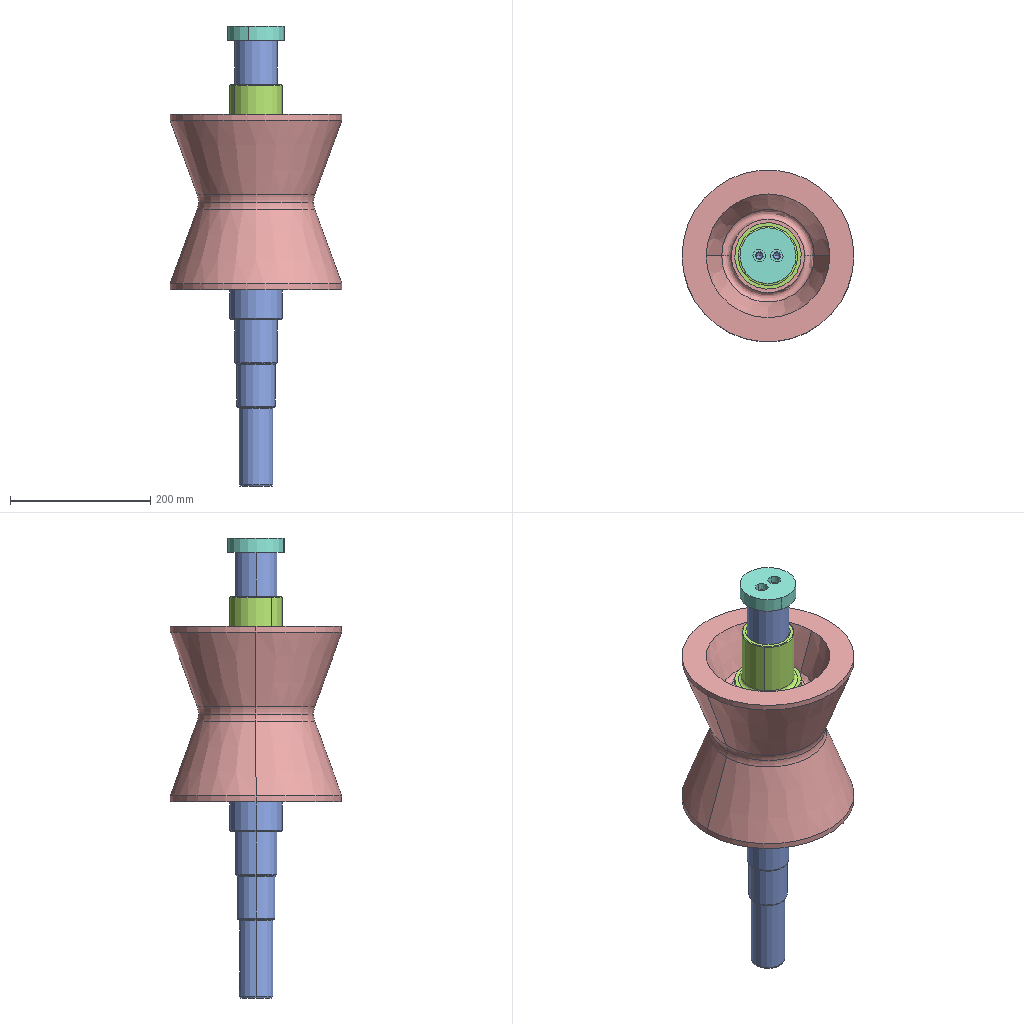Assembly | SolidWorks | 5 different items | 5 placed | box 245 x 244 x 656 mm
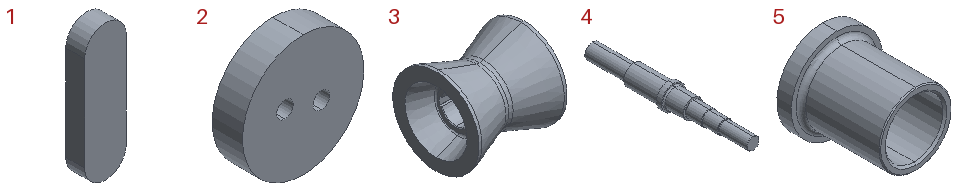Parts list (item | quantity | size | volume | features):
1 | x1 | 22 x 10 x 72 mm | 14801 mm3 | features Extrusion 1
2 | x1 | 80 x 20 x 80 mm | 93222 mm3 | features 3DProfileFeature 1, Extrusion 1, HoleWzd 1
3 | x1 | 250 x 245 x 245 mm | 5466955 mm3 | features Chamfer 1, Fillet 1, ICE 1, Revolution 1
4 | x1 | 95 x 636 x 95 mm | 2135437 mm3 | features Chamfer 4, Fillet 3, ICE 2, HoleWzd 1, Revolution 1
5 | x1 | 95 x 97 x 95 mm | 192640 mm3 | features Chamfer 3, Extrusion 1, Fillet 1, ICE 1
Mates (type | each side: item.copy, entity, surface, feature):
Concentric | 3.1 face cylinder Cut-Extrude1 | 4.1 face cylinder Revolve1
Coincident | 3.1 face plane Cut-Extrude1 | 4.1 face plane Cut-Extrude1
Coincident | 3.1 face plane Revolve1 | 4.1 face plane Revolve1
Concentric | 4.1 face cylinder Revolve1 | 5.1 face cylinder Boss-Extrude2
Coincident | 3.1 face plane Revolve1 | 5.1 face plane Boss-Extrude1
Coincident | 4.1 plane | assembly plane
Coincident | 4.1 face plane Cut-Extrude1 | 1.1 face plane Boss-Extrude1 | 2 times
Concentric | 4.1 face cylinder Revolve1 | 2.1 face cylinder Boss-Extrude1
Coincident | 4.1 face plane Revolve1 | 2.1 face plane Boss-Extrude1